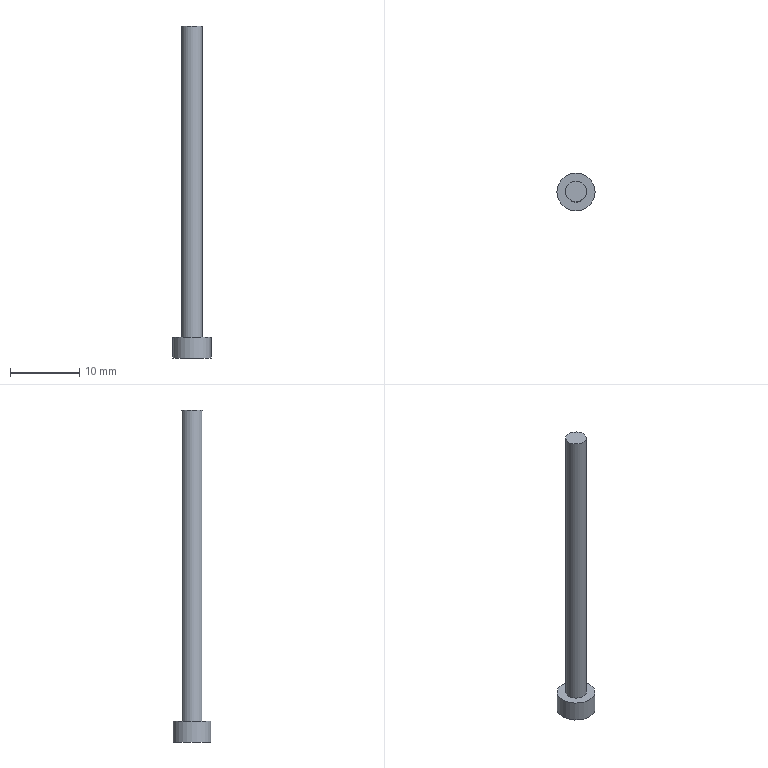Part | STEP file | 1 solid | 12 faces | box 5.5 x 5.5 x 48 mm | volume 378.644 mm3 | plane 10 | cylinder 2 | commonest cylinder face diameters 3 x1 5.5 x1
STEP:
#1=CARTESIAN_POINT('',(0.,0.,0.));
#2=DIRECTION('',(0.,0.,1.));
#3=DIRECTION('',(1.,0.,0.));
#4=AXIS2_PLACEMENT_3D('',#1,#2,#3);
#5=CARTESIAN_POINT('',(1805.407,450.23,-94.881));
#6=VERTEX_POINT('',#5);
#7=CARTESIAN_POINT('',(1808.157,450.23,-94.881));
#8=DIRECTION('',(0.,0.,-1.));
#9=DIRECTION('',(-1.,0.,0.));
#10=AXIS2_PLACEMENT_3D('',#7,#8,#9);
#11=CIRCLE('',#10,2.75);
#12=CARTESIAN_POINT('',(1805.407,450.23,-94.881));
#13=DIRECTION('',(0.,0.,1.));
#14=DIRECTION('',(1.,0.,0.));
#15=AXIS2_PLACEMENT_3D('',#12,#13,#14);
#16=PLANE('',#15);
#17=CARTESIAN_POINT('',(0.,0.));
#18=CARTESIAN_POINT('',(0.,4.763));
#19=CARTESIAN_POINT('',(4.125,2.382));
#20=CARTESIAN_POINT('',(8.25,0.));
#21=CARTESIAN_POINT('',(4.125,-2.382));
#22=CARTESIAN_POINT('',(0.,-4.763));
#23=CARTESIAN_POINT('',(0.,0.));
#24=(BOUNDED_CURVE()B_SPLINE_CURVE(2,(#17,#18,#19,#20,#21,#22,#23),.UNSPECIFIED.,.T.,.F.)B_SPLINE_CURVE_WITH_KNOTS((1,2,2,2,2,1),(-2.094,0.,2.094,4.189,6.283,8.378),.UNSPECIFIED.)CURVE()GEOMETRIC_REPRESENTATION_ITEM()RATIONAL_B_SPLINE_CURVE((1.,0.5,1.,0.5,1.,0.5,1.))REPRESENTATION_ITEM(''));
#25=(GEOMETRIC_REPRESENTATION_CONTEXT(2)PARAMETRIC_REPRESENTATION_CONTEXT()REPRESENTATION_CONTEXT('',''));
#26=DEFINITIONAL_REPRESENTATION('',(#24),#25);
#27=PCURVE('',#16,#26);
#28=CARTESIAN_POINT('',(1808.157,450.23,-52.481));
#29=DIRECTION('',(0.,0.,-1.));
#30=DIRECTION('',(-1.,0.,0.));
#31=AXIS2_PLACEMENT_3D('',#28,#29,#30);
#32=CYLINDRICAL_SURFACE('',#31,2.75);
#33=CARTESIAN_POINT('',(0.,42.4));
#34=DIRECTION('',(1.,0.));
#35=VECTOR('',#34,1.);
#36=LINE('',#33,#35);
#37=(GEOMETRIC_REPRESENTATION_CONTEXT(2)PARAMETRIC_REPRESENTATION_CONTEXT()REPRESENTATION_CONTEXT('',''));
#38=DEFINITIONAL_REPRESENTATION('',(#36),#37);
#39=PCURVE('',#32,#38);
#40=SURFACE_CURVE('',#11,(#27,#39),.PCURVE_S1.);
#41=EDGE_CURVE('',#6,#6,#40,.T.);
#42=ORIENTED_EDGE('',*,*,#41,.T.);
#43=EDGE_LOOP('',(#42));
#44=FACE_BOUND('',#43,.T.);
#45=CARTESIAN_POINT('',(1808.879,451.48,-94.881));
#46=VERTEX_POINT('',#45);
#47=CARTESIAN_POINT('',(1807.435,451.48,-94.881));
#48=VERTEX_POINT('',#47);
#49=CARTESIAN_POINT('',(1808.879,451.48,-94.881));
#50=DIRECTION('',(-1.,0.,0.));
#51=VECTOR('',#50,1.);
#52=LINE('',#49,#51);
#53=CARTESIAN_POINT('',(3.472,1.25));
#54=DIRECTION('',(-1.,0.));
#55=VECTOR('',#54,1.);
#56=LINE('',#53,#55);
#57=(GEOMETRIC_REPRESENTATION_CONTEXT(2)PARAMETRIC_REPRESENTATION_CONTEXT()REPRESENTATION_CONTEXT('',''));
#58=DEFINITIONAL_REPRESENTATION('',(#56),#57);
#59=PCURVE('',#16,#58);
#60=CARTESIAN_POINT('',(1808.879,451.48,-92.901));
#61=DIRECTION('',(0.,-1.,0.));
#62=DIRECTION('',(-1.,0.,0.));
#63=AXIS2_PLACEMENT_3D('',#60,#61,#62);
#64=PLANE('',#63);
#65=CARTESIAN_POINT('',(0.,1.98));
#66=DIRECTION('',(1.,0.));
#67=VECTOR('',#66,1.);
#68=LINE('',#65,#67);
#69=(GEOMETRIC_REPRESENTATION_CONTEXT(2)PARAMETRIC_REPRESENTATION_CONTEXT()REPRESENTATION_CONTEXT('',''));
#70=DEFINITIONAL_REPRESENTATION('',(#68),#69);
#71=PCURVE('',#64,#70);
#72=SURFACE_CURVE('',#52,(#59,#71),.PCURVE_S1.);
#73=EDGE_CURVE('',#46,#48,#72,.T.);
#74=ORIENTED_EDGE('',*,*,#73,.T.);
#75=CARTESIAN_POINT('',(1806.714,450.23,-94.881));
#76=VERTEX_POINT('',#75);
#77=CARTESIAN_POINT('',(1807.435,451.48,-94.881));
#78=DIRECTION('',(-0.5,-0.866,0.));
#79=VECTOR('',#78,1.);
#80=LINE('',#77,#79);
#81=CARTESIAN_POINT('',(2.028,1.25));
#82=DIRECTION('',(-0.5,-0.866));
#83=VECTOR('',#82,1.);
#84=LINE('',#81,#83);
#85=(GEOMETRIC_REPRESENTATION_CONTEXT(2)PARAMETRIC_REPRESENTATION_CONTEXT()REPRESENTATION_CONTEXT('',''));
#86=DEFINITIONAL_REPRESENTATION('',(#84),#85);
#87=PCURVE('',#16,#86);
#88=CARTESIAN_POINT('',(1807.435,451.48,-92.901));
#89=DIRECTION('',(0.866,-0.5,0.));
#90=DIRECTION('',(-0.5,-0.866,0.));
#91=AXIS2_PLACEMENT_3D('',#88,#89,#90);
#92=PLANE('',#91);
#93=CARTESIAN_POINT('',(0.,1.98));
#94=DIRECTION('',(1.,0.));
#95=VECTOR('',#94,1.);
#96=LINE('',#93,#95);
#97=(GEOMETRIC_REPRESENTATION_CONTEXT(2)PARAMETRIC_REPRESENTATION_CONTEXT()REPRESENTATION_CONTEXT('',''));
#98=DEFINITIONAL_REPRESENTATION('',(#96),#97);
#99=PCURVE('',#92,#98);
#100=SURFACE_CURVE('',#80,(#87,#99),.PCURVE_S1.);
#101=EDGE_CURVE('',#48,#76,#100,.T.);
#102=ORIENTED_EDGE('',*,*,#101,.T.);
#103=CARTESIAN_POINT('',(1807.435,448.98,-94.881));
#104=VERTEX_POINT('',#103);
#105=CARTESIAN_POINT('',(1806.714,450.23,-94.881));
#106=DIRECTION('',(0.5,-0.866,0.));
#107=VECTOR('',#106,1.);
#108=LINE('',#105,#107);
#109=CARTESIAN_POINT('',(1.307,0.));
#110=DIRECTION('',(0.5,-0.866));
#111=VECTOR('',#110,1.);
#112=LINE('',#109,#111);
#113=(GEOMETRIC_REPRESENTATION_CONTEXT(2)PARAMETRIC_REPRESENTATION_CONTEXT()REPRESENTATION_CONTEXT('',''));
#114=DEFINITIONAL_REPRESENTATION('',(#112),#113);
#115=PCURVE('',#16,#114);
#116=CARTESIAN_POINT('',(1806.714,450.23,-92.901));
#117=DIRECTION('',(0.866,0.5,0.));
#118=DIRECTION('',(0.5,-0.866,0.));
#119=AXIS2_PLACEMENT_3D('',#116,#117,#118);
#120=PLANE('',#119);
#121=CARTESIAN_POINT('',(0.,1.98));
#122=DIRECTION('',(1.,0.));
#123=VECTOR('',#122,1.);
#124=LINE('',#121,#123);
#125=(GEOMETRIC_REPRESENTATION_CONTEXT(2)PARAMETRIC_REPRESENTATION_CONTEXT()REPRESENTATION_CONTEXT('',''));
#126=DEFINITIONAL_REPRESENTATION('',(#124),#125);
#127=PCURVE('',#120,#126);
#128=SURFACE_CURVE('',#108,(#115,#127),.PCURVE_S1.);
#129=EDGE_CURVE('',#76,#104,#128,.T.);
#130=ORIENTED_EDGE('',*,*,#129,.T.);
#131=CARTESIAN_POINT('',(1808.879,448.98,-94.881));
#132=VERTEX_POINT('',#131);
#133=CARTESIAN_POINT('',(1807.435,448.98,-94.881));
#134=DIRECTION('',(1.,0.,0.));
#135=VECTOR('',#134,1.);
#136=LINE('',#133,#135);
#137=CARTESIAN_POINT('',(2.028,-1.25));
#138=DIRECTION('',(1.,0.));
#139=VECTOR('',#138,1.);
#140=LINE('',#137,#139);
#141=(GEOMETRIC_REPRESENTATION_CONTEXT(2)PARAMETRIC_REPRESENTATION_CONTEXT()REPRESENTATION_CONTEXT('',''));
#142=DEFINITIONAL_REPRESENTATION('',(#140),#141);
#143=PCURVE('',#16,#142);
#144=CARTESIAN_POINT('',(1807.435,448.98,-92.901));
#145=DIRECTION('',(0.,1.,0.));
#146=DIRECTION('',(1.,0.,0.));
#147=AXIS2_PLACEMENT_3D('',#144,#145,#146);
#148=PLANE('',#147);
#149=CARTESIAN_POINT('',(0.,1.98));
#150=DIRECTION('',(1.,0.));
#151=VECTOR('',#150,1.);
#152=LINE('',#149,#151);
#153=(GEOMETRIC_REPRESENTATION_CONTEXT(2)PARAMETRIC_REPRESENTATION_CONTEXT()REPRESENTATION_CONTEXT('',''));
#154=DEFINITIONAL_REPRESENTATION('',(#152),#153);
#155=PCURVE('',#148,#154);
#156=SURFACE_CURVE('',#136,(#143,#155),.PCURVE_S1.);
#157=EDGE_CURVE('',#104,#132,#156,.T.);
#158=ORIENTED_EDGE('',*,*,#157,.T.);
#159=CARTESIAN_POINT('',(1809.601,450.23,-94.881));
#160=VERTEX_POINT('',#159);
#161=CARTESIAN_POINT('',(1808.879,448.98,-94.881));
#162=DIRECTION('',(0.5,0.866,0.));
#163=VECTOR('',#162,1.);
#164=LINE('',#161,#163);
#165=CARTESIAN_POINT('',(3.472,-1.25));
#166=DIRECTION('',(0.5,0.866));
#167=VECTOR('',#166,1.);
#168=LINE('',#165,#167);
#169=(GEOMETRIC_REPRESENTATION_CONTEXT(2)PARAMETRIC_REPRESENTATION_CONTEXT()REPRESENTATION_CONTEXT('',''));
#170=DEFINITIONAL_REPRESENTATION('',(#168),#169);
#171=PCURVE('',#16,#170);
#172=CARTESIAN_POINT('',(1808.879,448.98,-92.901));
#173=DIRECTION('',(-0.866,0.5,0.));
#174=DIRECTION('',(0.5,0.866,0.));
#175=AXIS2_PLACEMENT_3D('',#172,#173,#174);
#176=PLANE('',#175);
#177=CARTESIAN_POINT('',(0.,1.98));
#178=DIRECTION('',(1.,0.));
#179=VECTOR('',#178,1.);
#180=LINE('',#177,#179);
#181=(GEOMETRIC_REPRESENTATION_CONTEXT(2)PARAMETRIC_REPRESENTATION_CONTEXT()REPRESENTATION_CONTEXT('',''));
#182=DEFINITIONAL_REPRESENTATION('',(#180),#181);
#183=PCURVE('',#176,#182);
#184=SURFACE_CURVE('',#164,(#171,#183),.PCURVE_S1.);
#185=EDGE_CURVE('',#132,#160,#184,.T.);
#186=ORIENTED_EDGE('',*,*,#185,.T.);
#187=CARTESIAN_POINT('',(1809.601,450.23,-94.881));
#188=DIRECTION('',(-0.5,0.866,0.));
#189=VECTOR('',#188,1.);
#190=LINE('',#187,#189);
#191=CARTESIAN_POINT('',(4.193,0.));
#192=DIRECTION('',(-0.5,0.866));
#193=VECTOR('',#192,1.);
#194=LINE('',#191,#193);
#195=(GEOMETRIC_REPRESENTATION_CONTEXT(2)PARAMETRIC_REPRESENTATION_CONTEXT()REPRESENTATION_CONTEXT('',''));
#196=DEFINITIONAL_REPRESENTATION('',(#194),#195);
#197=PCURVE('',#16,#196);
#198=CARTESIAN_POINT('',(1809.601,450.23,-92.901));
#199=DIRECTION('',(-0.866,-0.5,0.));
#200=DIRECTION('',(-0.5,0.866,0.));
#201=AXIS2_PLACEMENT_3D('',#198,#199,#200);
#202=PLANE('',#201);
#203=CARTESIAN_POINT('',(0.,1.98));
#204=DIRECTION('',(1.,0.));
#205=VECTOR('',#204,1.);
#206=LINE('',#203,#205);
#207=(GEOMETRIC_REPRESENTATION_CONTEXT(2)PARAMETRIC_REPRESENTATION_CONTEXT()REPRESENTATION_CONTEXT('',''));
#208=DEFINITIONAL_REPRESENTATION('',(#206),#207);
#209=PCURVE('',#202,#208);
#210=SURFACE_CURVE('',#190,(#197,#209),.PCURVE_S1.);
#211=EDGE_CURVE('',#160,#46,#210,.T.);
#212=ORIENTED_EDGE('',*,*,#211,.T.);
#213=EDGE_LOOP('',(#74,#102,#130,#158,#186,#212));
#214=FACE_BOUND('',#213,.T.);
#215=ADVANCED_FACE('',(#44,#214),#16,.F.);
#216=ORIENTED_EDGE('',*,*,#41,.F.);
#217=CARTESIAN_POINT('',(1805.407,450.23,-91.881));
#218=VERTEX_POINT('',#217);
#219=CARTESIAN_POINT('',(1805.407,450.23,-91.881));
#220=CARTESIAN_POINT('',(1805.407,450.23,-94.881));
#221=B_SPLINE_CURVE_WITH_KNOTS('',1,(#219,#220),.UNSPECIFIED.,.F.,.F.,(2,2),(39.4,42.4),.PIECEWISE_BEZIER_KNOTS.);
#222=CARTESIAN_POINT('',(0.,0.));
#223=DIRECTION('',(0.,1.));
#224=VECTOR('',#223,1.);
#225=LINE('',#222,#224);
#226=(GEOMETRIC_REPRESENTATION_CONTEXT(2)PARAMETRIC_REPRESENTATION_CONTEXT()REPRESENTATION_CONTEXT('',''));
#227=DEFINITIONAL_REPRESENTATION('',(#225),#226);
#228=PCURVE('',#32,#227);
#229=CARTESIAN_POINT('',(6.283,0.));
#230=DIRECTION('',(0.,1.));
#231=VECTOR('',#230,1.);
#232=LINE('',#229,#231);
#233=(GEOMETRIC_REPRESENTATION_CONTEXT(2)PARAMETRIC_REPRESENTATION_CONTEXT()REPRESENTATION_CONTEXT('',''));
#234=DEFINITIONAL_REPRESENTATION('',(#232),#233);
#235=PCURVE('',#32,#234);
#236=SEAM_CURVE('',#221,(#228,#235),.PCURVE_S1.);
#237=EDGE_CURVE('',#218,#6,#236,.T.);
#238=ORIENTED_EDGE('',*,*,#237,.F.);
#239=CARTESIAN_POINT('',(1808.157,450.23,-91.881));
#240=DIRECTION('',(0.,0.,-1.));
#241=DIRECTION('',(-1.,0.,0.));
#242=AXIS2_PLACEMENT_3D('',#239,#240,#241);
#243=CIRCLE('',#242,2.75);
#244=CARTESIAN_POINT('',(0.,39.4));
#245=DIRECTION('',(1.,0.));
#246=VECTOR('',#245,1.);
#247=LINE('',#244,#246);
#248=(GEOMETRIC_REPRESENTATION_CONTEXT(2)PARAMETRIC_REPRESENTATION_CONTEXT()REPRESENTATION_CONTEXT('',''));
#249=DEFINITIONAL_REPRESENTATION('',(#247),#248);
#250=PCURVE('',#32,#249);
#251=CARTESIAN_POINT('',(1806.657,450.23,-91.881));
#252=DIRECTION('',(0.,0.,-1.));
#253=DIRECTION('',(-1.,0.,0.));
#254=AXIS2_PLACEMENT_3D('',#251,#252,#253);
#255=PLANE('',#254);
#256=CARTESIAN_POINT('',(-1.5,0.));
#257=DIRECTION('',(1.,0.));
#258=AXIS2_PLACEMENT_2D('',#256,#257);
#259=CIRCLE('',#258,2.75);
#260=(GEOMETRIC_REPRESENTATION_CONTEXT(2)PARAMETRIC_REPRESENTATION_CONTEXT()REPRESENTATION_CONTEXT('',''));
#261=DEFINITIONAL_REPRESENTATION('',(#259),#260);
#262=PCURVE('',#255,#261);
#263=SURFACE_CURVE('',#243,(#250,#262),.PCURVE_S1.);
#264=EDGE_CURVE('',#218,#218,#263,.T.);
#265=ORIENTED_EDGE('',*,*,#264,.T.);
#266=ORIENTED_EDGE('',*,*,#237,.T.);
#267=EDGE_LOOP('',(#216,#238,#265,#266));
#268=FACE_BOUND('',#267,.T.);
#269=ADVANCED_FACE('',(#268),#32,.T.);
#270=ORIENTED_EDGE('',*,*,#264,.F.);
#271=EDGE_LOOP('',(#270));
#272=FACE_BOUND('',#271,.T.);
#273=CARTESIAN_POINT('',(1806.657,450.23,-91.881));
#274=VERTEX_POINT('',#273);
#275=CARTESIAN_POINT('',(1808.157,450.23,-91.881));
#276=DIRECTION('',(0.,0.,-1.));
#277=DIRECTION('',(-1.,0.,0.));
#278=AXIS2_PLACEMENT_3D('',#275,#276,#277);
#279=CIRCLE('',#278,1.5);
#280=CARTESIAN_POINT('',(-1.5,0.));
#281=DIRECTION('',(1.,0.));
#282=AXIS2_PLACEMENT_2D('',#280,#281);
#283=CIRCLE('',#282,1.5);
#284=(GEOMETRIC_REPRESENTATION_CONTEXT(2)PARAMETRIC_REPRESENTATION_CONTEXT()REPRESENTATION_CONTEXT('',''));
#285=DEFINITIONAL_REPRESENTATION('',(#283),#284);
#286=PCURVE('',#255,#285);
#287=CARTESIAN_POINT('',(1808.157,450.23,-52.481));
#288=DIRECTION('',(0.,0.,-1.));
#289=DIRECTION('',(-1.,0.,0.));
#290=AXIS2_PLACEMENT_3D('',#287,#288,#289);
#291=CYLINDRICAL_SURFACE('',#290,1.5);
#292=CARTESIAN_POINT('',(0.,39.4));
#293=DIRECTION('',(1.,0.));
#294=VECTOR('',#293,1.);
#295=LINE('',#292,#294);
#296=(GEOMETRIC_REPRESENTATION_CONTEXT(2)PARAMETRIC_REPRESENTATION_CONTEXT()REPRESENTATION_CONTEXT('',''));
#297=DEFINITIONAL_REPRESENTATION('',(#295),#296);
#298=PCURVE('',#291,#297);
#299=SURFACE_CURVE('',#279,(#286,#298),.PCURVE_S1.);
#300=EDGE_CURVE('',#274,#274,#299,.T.);
#301=ORIENTED_EDGE('',*,*,#300,.T.);
#302=EDGE_LOOP('',(#301));
#303=FACE_BOUND('',#302,.T.);
#304=ADVANCED_FACE('',(#272,#303),#255,.F.);
#305=ORIENTED_EDGE('',*,*,#300,.F.);
#306=CARTESIAN_POINT('',(1806.657,450.23,-46.881));
#307=VERTEX_POINT('',#306);
#308=CARTESIAN_POINT('',(1806.657,450.23,-46.881));
#309=CARTESIAN_POINT('',(1806.657,450.23,-91.881));
#310=B_SPLINE_CURVE_WITH_KNOTS('',1,(#308,#309),.UNSPECIFIED.,.F.,.F.,(2,2),(-5.6,39.4),.PIECEWISE_BEZIER_KNOTS.);
#311=CARTESIAN_POINT('',(0.,0.));
#312=DIRECTION('',(0.,1.));
#313=VECTOR('',#312,1.);
#314=LINE('',#311,#313);
#315=(GEOMETRIC_REPRESENTATION_CONTEXT(2)PARAMETRIC_REPRESENTATION_CONTEXT()REPRESENTATION_CONTEXT('',''));
#316=DEFINITIONAL_REPRESENTATION('',(#314),#315);
#317=PCURVE('',#291,#316);
#318=CARTESIAN_POINT('',(6.283,0.));
#319=DIRECTION('',(0.,1.));
#320=VECTOR('',#319,1.);
#321=LINE('',#318,#320);
#322=(GEOMETRIC_REPRESENTATION_CONTEXT(2)PARAMETRIC_REPRESENTATION_CONTEXT()REPRESENTATION_CONTEXT('',''));
#323=DEFINITIONAL_REPRESENTATION('',(#321),#322);
#324=PCURVE('',#291,#323);
#325=SEAM_CURVE('',#310,(#317,#324),.PCURVE_S1.);
#326=EDGE_CURVE('',#307,#274,#325,.T.);
#327=ORIENTED_EDGE('',*,*,#326,.F.);
#328=CARTESIAN_POINT('',(1808.157,450.23,-46.881));
#329=DIRECTION('',(0.,0.,-1.));
#330=DIRECTION('',(-1.,0.,0.));
#331=AXIS2_PLACEMENT_3D('',#328,#329,#330);
#332=CIRCLE('',#331,1.5);
#333=CARTESIAN_POINT('',(0.,-5.6));
#334=DIRECTION('',(1.,0.));
#335=VECTOR('',#334,1.);
#336=LINE('',#333,#335);
#337=(GEOMETRIC_REPRESENTATION_CONTEXT(2)PARAMETRIC_REPRESENTATION_CONTEXT()REPRESENTATION_CONTEXT('',''));
#338=DEFINITIONAL_REPRESENTATION('',(#336),#337);
#339=PCURVE('',#291,#338);
#340=CARTESIAN_POINT('',(1808.157,450.23,-46.881));
#341=DIRECTION('',(0.,0.,-1.));
#342=DIRECTION('',(-1.,0.,0.));
#343=AXIS2_PLACEMENT_3D('',#340,#341,#342);
#344=PLANE('',#343);
#345=CARTESIAN_POINT('',(0.,0.));
#346=DIRECTION('',(1.,0.));
#347=AXIS2_PLACEMENT_2D('',#345,#346);
#348=CIRCLE('',#347,1.5);
#349=(GEOMETRIC_REPRESENTATION_CONTEXT(2)PARAMETRIC_REPRESENTATION_CONTEXT()REPRESENTATION_CONTEXT('',''));
#350=DEFINITIONAL_REPRESENTATION('',(#348),#349);
#351=PCURVE('',#344,#350);
#352=SURFACE_CURVE('',#332,(#339,#351),.PCURVE_S1.);
#353=EDGE_CURVE('',#307,#307,#352,.T.);
#354=ORIENTED_EDGE('',*,*,#353,.T.);
#355=ORIENTED_EDGE('',*,*,#326,.T.);
#356=EDGE_LOOP('',(#305,#327,#354,#355));
#357=FACE_BOUND('',#356,.T.);
#358=ADVANCED_FACE('',(#357),#291,.T.);
#359=ORIENTED_EDGE('',*,*,#353,.F.);
#360=EDGE_LOOP('',(#359));
#361=FACE_BOUND('',#360,.T.);
#362=ADVANCED_FACE('',(#361),#344,.F.);
#363=ORIENTED_EDGE('',*,*,#73,.F.);
#364=CARTESIAN_POINT('',(1808.879,451.48,-92.901));
#365=VERTEX_POINT('',#364);
#366=CARTESIAN_POINT('',(1808.879,451.48,-92.901));
#367=DIRECTION('',(0.,0.,1.));
#368=VECTOR('',#367,1.);
#369=LINE('',#366,#368);
#370=CARTESIAN_POINT('',(0.,0.));
#371=DIRECTION('',(0.,-1.));
#372=VECTOR('',#371,1.);
#373=LINE('',#370,#372);
#374=(GEOMETRIC_REPRESENTATION_CONTEXT(2)PARAMETRIC_REPRESENTATION_CONTEXT()REPRESENTATION_CONTEXT('',''));
#375=DEFINITIONAL_REPRESENTATION('',(#373),#374);
#376=PCURVE('',#64,#375);
#377=CARTESIAN_POINT('',(1.443,0.));
#378=DIRECTION('',(0.,-1.));
#379=VECTOR('',#378,1.);
#380=LINE('',#377,#379);
#381=(GEOMETRIC_REPRESENTATION_CONTEXT(2)PARAMETRIC_REPRESENTATION_CONTEXT()REPRESENTATION_CONTEXT('',''));
#382=DEFINITIONAL_REPRESENTATION('',(#380),#381);
#383=PCURVE('',#202,#382);
#384=SURFACE_CURVE('',#369,(#376,#383),.PCURVE_S1.);
#385=EDGE_CURVE('',#46,#365,#384,.T.);
#386=ORIENTED_EDGE('',*,*,#385,.T.);
#387=CARTESIAN_POINT('',(1807.435,451.48,-92.901));
#388=VERTEX_POINT('',#387);
#389=CARTESIAN_POINT('',(1808.879,451.48,-92.901));
#390=DIRECTION('',(1.,0.,0.));
#391=VECTOR('',#390,1.);
#392=LINE('',#389,#391);
#393=CARTESIAN_POINT('',(0.,0.));
#394=DIRECTION('',(-1.,0.));
#395=VECTOR('',#394,1.);
#396=LINE('',#393,#395);
#397=(GEOMETRIC_REPRESENTATION_CONTEXT(2)PARAMETRIC_REPRESENTATION_CONTEXT()REPRESENTATION_CONTEXT('',''));
#398=DEFINITIONAL_REPRESENTATION('',(#396),#397);
#399=PCURVE('',#64,#398);
#400=CARTESIAN_POINT('',(1808.157,450.23,-92.901));
#401=DIRECTION('',(0.,0.,1.));
#402=DIRECTION('',(1.,0.,0.));
#403=AXIS2_PLACEMENT_3D('',#400,#401,#402);
#404=PLANE('',#403);
#405=CARTESIAN_POINT('',(0.7217,1.25));
#406=DIRECTION('',(1.,0.));
#407=VECTOR('',#406,1.);
#408=LINE('',#405,#407);
#409=(GEOMETRIC_REPRESENTATION_CONTEXT(2)PARAMETRIC_REPRESENTATION_CONTEXT()REPRESENTATION_CONTEXT('',''));
#410=DEFINITIONAL_REPRESENTATION('',(#408),#409);
#411=PCURVE('',#404,#410);
#412=SURFACE_CURVE('',#392,(#399,#411),.PCURVE_S1.);
#413=EDGE_CURVE('',#388,#365,#412,.T.);
#414=ORIENTED_EDGE('',*,*,#413,.F.);
#415=CARTESIAN_POINT('',(1807.435,451.48,-92.901));
#416=DIRECTION('',(0.,0.,1.));
#417=VECTOR('',#416,1.);
#418=LINE('',#415,#417);
#419=CARTESIAN_POINT('',(1.443,0.));
#420=DIRECTION('',(0.,-1.));
#421=VECTOR('',#420,1.);
#422=LINE('',#419,#421);
#423=(GEOMETRIC_REPRESENTATION_CONTEXT(2)PARAMETRIC_REPRESENTATION_CONTEXT()REPRESENTATION_CONTEXT('',''));
#424=DEFINITIONAL_REPRESENTATION('',(#422),#423);
#425=PCURVE('',#64,#424);
#426=CARTESIAN_POINT('',(0.,0.));
#427=DIRECTION('',(0.,-1.));
#428=VECTOR('',#427,1.);
#429=LINE('',#426,#428);
#430=(GEOMETRIC_REPRESENTATION_CONTEXT(2)PARAMETRIC_REPRESENTATION_CONTEXT()REPRESENTATION_CONTEXT('',''));
#431=DEFINITIONAL_REPRESENTATION('',(#429),#430);
#432=PCURVE('',#92,#431);
#433=SURFACE_CURVE('',#418,(#425,#432),.PCURVE_S1.);
#434=EDGE_CURVE('',#48,#388,#433,.T.);
#435=ORIENTED_EDGE('',*,*,#434,.F.);
#436=EDGE_LOOP('',(#363,#386,#414,#435));
#437=FACE_BOUND('',#436,.T.);
#438=ADVANCED_FACE('',(#437),#64,.T.);
#439=ORIENTED_EDGE('',*,*,#101,.F.);
#440=ORIENTED_EDGE('',*,*,#434,.T.);
#441=CARTESIAN_POINT('',(1806.714,450.23,-92.901));
#442=VERTEX_POINT('',#441);
#443=CARTESIAN_POINT('',(1807.435,451.48,-92.901));
#444=DIRECTION('',(0.5,0.866,0.));
#445=VECTOR('',#444,1.);
#446=LINE('',#443,#445);
#447=CARTESIAN_POINT('',(0.,0.));
#448=DIRECTION('',(-1.,0.));
#449=VECTOR('',#448,1.);
#450=LINE('',#447,#449);
#451=(GEOMETRIC_REPRESENTATION_CONTEXT(2)PARAMETRIC_REPRESENTATION_CONTEXT()REPRESENTATION_CONTEXT('',''));
#452=DEFINITIONAL_REPRESENTATION('',(#450),#451);
#453=PCURVE('',#92,#452);
#454=CARTESIAN_POINT('',(-0.7217,1.25));
#455=DIRECTION('',(0.5,0.866));
#456=VECTOR('',#455,1.);
#457=LINE('',#454,#456);
#458=(GEOMETRIC_REPRESENTATION_CONTEXT(2)PARAMETRIC_REPRESENTATION_CONTEXT()REPRESENTATION_CONTEXT('',''));
#459=DEFINITIONAL_REPRESENTATION('',(#457),#458);
#460=PCURVE('',#404,#459);
#461=SURFACE_CURVE('',#446,(#453,#460),.PCURVE_S1.);
#462=EDGE_CURVE('',#442,#388,#461,.T.);
#463=ORIENTED_EDGE('',*,*,#462,.F.);
#464=CARTESIAN_POINT('',(1806.714,450.23,-92.901));
#465=DIRECTION('',(0.,0.,1.));
#466=VECTOR('',#465,1.);
#467=LINE('',#464,#466);
#468=CARTESIAN_POINT('',(1.443,0.));
#469=DIRECTION('',(0.,-1.));
#470=VECTOR('',#469,1.);
#471=LINE('',#468,#470);
#472=(GEOMETRIC_REPRESENTATION_CONTEXT(2)PARAMETRIC_REPRESENTATION_CONTEXT()REPRESENTATION_CONTEXT('',''));
#473=DEFINITIONAL_REPRESENTATION('',(#471),#472);
#474=PCURVE('',#92,#473);
#475=CARTESIAN_POINT('',(0.,0.));
#476=DIRECTION('',(0.,-1.));
#477=VECTOR('',#476,1.);
#478=LINE('',#475,#477);
#479=(GEOMETRIC_REPRESENTATION_CONTEXT(2)PARAMETRIC_REPRESENTATION_CONTEXT()REPRESENTATION_CONTEXT('',''));
#480=DEFINITIONAL_REPRESENTATION('',(#478),#479);
#481=PCURVE('',#120,#480);
#482=SURFACE_CURVE('',#467,(#474,#481),.PCURVE_S1.);
#483=EDGE_CURVE('',#76,#442,#482,.T.);
#484=ORIENTED_EDGE('',*,*,#483,.F.);
#485=EDGE_LOOP('',(#439,#440,#463,#484));
#486=FACE_BOUND('',#485,.T.);
#487=ADVANCED_FACE('',(#486),#92,.T.);
#488=ORIENTED_EDGE('',*,*,#129,.F.);
#489=ORIENTED_EDGE('',*,*,#483,.T.);
#490=CARTESIAN_POINT('',(1807.435,448.98,-92.901));
#491=VERTEX_POINT('',#490);
#492=CARTESIAN_POINT('',(1806.714,450.23,-92.901));
#493=DIRECTION('',(-0.5,0.866,0.));
#494=VECTOR('',#493,1.);
#495=LINE('',#492,#494);
#496=CARTESIAN_POINT('',(0.,0.));
#497=DIRECTION('',(-1.,0.));
#498=VECTOR('',#497,1.);
#499=LINE('',#496,#498);
#500=(GEOMETRIC_REPRESENTATION_CONTEXT(2)PARAMETRIC_REPRESENTATION_CONTEXT()REPRESENTATION_CONTEXT('',''));
#501=DEFINITIONAL_REPRESENTATION('',(#499),#500);
#502=PCURVE('',#120,#501);
#503=CARTESIAN_POINT('',(-1.443,0.));
#504=DIRECTION('',(-0.5,0.866));
#505=VECTOR('',#504,1.);
#506=LINE('',#503,#505);
#507=(GEOMETRIC_REPRESENTATION_CONTEXT(2)PARAMETRIC_REPRESENTATION_CONTEXT()REPRESENTATION_CONTEXT('',''));
#508=DEFINITIONAL_REPRESENTATION('',(#506),#507);
#509=PCURVE('',#404,#508);
#510=SURFACE_CURVE('',#495,(#502,#509),.PCURVE_S1.);
#511=EDGE_CURVE('',#491,#442,#510,.T.);
#512=ORIENTED_EDGE('',*,*,#511,.F.);
#513=CARTESIAN_POINT('',(1807.435,448.98,-92.901));
#514=DIRECTION('',(0.,0.,1.));
#515=VECTOR('',#514,1.);
#516=LINE('',#513,#515);
#517=CARTESIAN_POINT('',(1.443,0.));
#518=DIRECTION('',(0.,-1.));
#519=VECTOR('',#518,1.);
#520=LINE('',#517,#519);
#521=(GEOMETRIC_REPRESENTATION_CONTEXT(2)PARAMETRIC_REPRESENTATION_CONTEXT()REPRESENTATION_CONTEXT('',''));
#522=DEFINITIONAL_REPRESENTATION('',(#520),#521);
#523=PCURVE('',#120,#522);
#524=CARTESIAN_POINT('',(0.,0.));
#525=DIRECTION('',(0.,-1.));
#526=VECTOR('',#525,1.);
#527=LINE('',#524,#526);
#528=(GEOMETRIC_REPRESENTATION_CONTEXT(2)PARAMETRIC_REPRESENTATION_CONTEXT()REPRESENTATION_CONTEXT('',''));
#529=DEFINITIONAL_REPRESENTATION('',(#527),#528);
#530=PCURVE('',#148,#529);
#531=SURFACE_CURVE('',#516,(#523,#530),.PCURVE_S1.);
#532=EDGE_CURVE('',#104,#491,#531,.T.);
#533=ORIENTED_EDGE('',*,*,#532,.F.);
#534=EDGE_LOOP('',(#488,#489,#512,#533));
#535=FACE_BOUND('',#534,.T.);
#536=ADVANCED_FACE('',(#535),#120,.T.);
#537=ORIENTED_EDGE('',*,*,#157,.F.);
#538=ORIENTED_EDGE('',*,*,#532,.T.);
#539=CARTESIAN_POINT('',(1808.879,448.98,-92.901));
#540=VERTEX_POINT('',#539);
#541=CARTESIAN_POINT('',(1807.435,448.98,-92.901));
#542=DIRECTION('',(-1.,0.,0.));
#543=VECTOR('',#542,1.);
#544=LINE('',#541,#543);
#545=CARTESIAN_POINT('',(0.,0.));
#546=DIRECTION('',(-1.,0.));
#547=VECTOR('',#546,1.);
#548=LINE('',#545,#547);
#549=(GEOMETRIC_REPRESENTATION_CONTEXT(2)PARAMETRIC_REPRESENTATION_CONTEXT()REPRESENTATION_CONTEXT('',''));
#550=DEFINITIONAL_REPRESENTATION('',(#548),#549);
#551=PCURVE('',#148,#550);
#552=CARTESIAN_POINT('',(-0.7217,-1.25));
#553=DIRECTION('',(-1.,0.));
#554=VECTOR('',#553,1.);
#555=LINE('',#552,#554);
#556=(GEOMETRIC_REPRESENTATION_CONTEXT(2)PARAMETRIC_REPRESENTATION_CONTEXT()REPRESENTATION_CONTEXT('',''));
#557=DEFINITIONAL_REPRESENTATION('',(#555),#556);
#558=PCURVE('',#404,#557);
#559=SURFACE_CURVE('',#544,(#551,#558),.PCURVE_S1.);
#560=EDGE_CURVE('',#540,#491,#559,.T.);
#561=ORIENTED_EDGE('',*,*,#560,.F.);
#562=CARTESIAN_POINT('',(1808.879,448.98,-92.901));
#563=DIRECTION('',(0.,0.,1.));
#564=VECTOR('',#563,1.);
#565=LINE('',#562,#564);
#566=CARTESIAN_POINT('',(1.443,0.));
#567=DIRECTION('',(0.,-1.));
#568=VECTOR('',#567,1.);
#569=LINE('',#566,#568);
#570=(GEOMETRIC_REPRESENTATION_CONTEXT(2)PARAMETRIC_REPRESENTATION_CONTEXT()REPRESENTATION_CONTEXT('',''));
#571=DEFINITIONAL_REPRESENTATION('',(#569),#570);
#572=PCURVE('',#148,#571);
#573=CARTESIAN_POINT('',(0.,0.));
#574=DIRECTION('',(0.,-1.));
#575=VECTOR('',#574,1.);
#576=LINE('',#573,#575);
#577=(GEOMETRIC_REPRESENTATION_CONTEXT(2)PARAMETRIC_REPRESENTATION_CONTEXT()REPRESENTATION_CONTEXT('',''));
#578=DEFINITIONAL_REPRESENTATION('',(#576),#577);
#579=PCURVE('',#176,#578);
#580=SURFACE_CURVE('',#565,(#572,#579),.PCURVE_S1.);
#581=EDGE_CURVE('',#132,#540,#580,.T.);
#582=ORIENTED_EDGE('',*,*,#581,.F.);
#583=EDGE_LOOP('',(#537,#538,#561,#582));
#584=FACE_BOUND('',#583,.T.);
#585=ADVANCED_FACE('',(#584),#148,.T.);
#586=ORIENTED_EDGE('',*,*,#185,.F.);
#587=ORIENTED_EDGE('',*,*,#581,.T.);
#588=CARTESIAN_POINT('',(1809.601,450.23,-92.901));
#589=VERTEX_POINT('',#588);
#590=CARTESIAN_POINT('',(1808.879,448.98,-92.901));
#591=DIRECTION('',(-0.5,-0.866,0.));
#592=VECTOR('',#591,1.);
#593=LINE('',#590,#592);
#594=CARTESIAN_POINT('',(0.,0.));
#595=DIRECTION('',(-1.,0.));
#596=VECTOR('',#595,1.);
#597=LINE('',#594,#596);
#598=(GEOMETRIC_REPRESENTATION_CONTEXT(2)PARAMETRIC_REPRESENTATION_CONTEXT()REPRESENTATION_CONTEXT('',''));
#599=DEFINITIONAL_REPRESENTATION('',(#597),#598);
#600=PCURVE('',#176,#599);
#601=CARTESIAN_POINT('',(0.7217,-1.25));
#602=DIRECTION('',(-0.5,-0.866));
#603=VECTOR('',#602,1.);
#604=LINE('',#601,#603);
#605=(GEOMETRIC_REPRESENTATION_CONTEXT(2)PARAMETRIC_REPRESENTATION_CONTEXT()REPRESENTATION_CONTEXT('',''));
#606=DEFINITIONAL_REPRESENTATION('',(#604),#605);
#607=PCURVE('',#404,#606);
#608=SURFACE_CURVE('',#593,(#600,#607),.PCURVE_S1.);
#609=EDGE_CURVE('',#589,#540,#608,.T.);
#610=ORIENTED_EDGE('',*,*,#609,.F.);
#611=CARTESIAN_POINT('',(1809.601,450.23,-92.901));
#612=DIRECTION('',(0.,0.,1.));
#613=VECTOR('',#612,1.);
#614=LINE('',#611,#613);
#615=CARTESIAN_POINT('',(1.443,0.));
#616=DIRECTION('',(0.,-1.));
#617=VECTOR('',#616,1.);
#618=LINE('',#615,#617);
#619=(GEOMETRIC_REPRESENTATION_CONTEXT(2)PARAMETRIC_REPRESENTATION_CONTEXT()REPRESENTATION_CONTEXT('',''));
#620=DEFINITIONAL_REPRESENTATION('',(#618),#619);
#621=PCURVE('',#176,#620);
#622=CARTESIAN_POINT('',(0.,0.));
#623=DIRECTION('',(0.,-1.));
#624=VECTOR('',#623,1.);
#625=LINE('',#622,#624);
#626=(GEOMETRIC_REPRESENTATION_CONTEXT(2)PARAMETRIC_REPRESENTATION_CONTEXT()REPRESENTATION_CONTEXT('',''));
#627=DEFINITIONAL_REPRESENTATION('',(#625),#626);
#628=PCURVE('',#202,#627);
#629=SURFACE_CURVE('',#614,(#621,#628),.PCURVE_S1.);
#630=EDGE_CURVE('',#160,#589,#629,.T.);
#631=ORIENTED_EDGE('',*,*,#630,.F.);
#632=EDGE_LOOP('',(#586,#587,#610,#631));
#633=FACE_BOUND('',#632,.T.);
#634=ADVANCED_FACE('',(#633),#176,.T.);
#635=ORIENTED_EDGE('',*,*,#211,.F.);
#636=ORIENTED_EDGE('',*,*,#630,.T.);
#637=CARTESIAN_POINT('',(1809.601,450.23,-92.901));
#638=DIRECTION('',(0.5,-0.866,0.));
#639=VECTOR('',#638,1.);
#640=LINE('',#637,#639);
#641=CARTESIAN_POINT('',(0.,0.));
#642=DIRECTION('',(-1.,0.));
#643=VECTOR('',#642,1.);
#644=LINE('',#641,#643);
#645=(GEOMETRIC_REPRESENTATION_CONTEXT(2)PARAMETRIC_REPRESENTATION_CONTEXT()REPRESENTATION_CONTEXT('',''));
#646=DEFINITIONAL_REPRESENTATION('',(#644),#645);
#647=PCURVE('',#202,#646);
#648=CARTESIAN_POINT('',(1.443,0.));
#649=DIRECTION('',(0.5,-0.866));
#650=VECTOR('',#649,1.);
#651=LINE('',#648,#650);
#652=(GEOMETRIC_REPRESENTATION_CONTEXT(2)PARAMETRIC_REPRESENTATION_CONTEXT()REPRESENTATION_CONTEXT('',''));
#653=DEFINITIONAL_REPRESENTATION('',(#651),#652);
#654=PCURVE('',#404,#653);
#655=SURFACE_CURVE('',#640,(#647,#654),.PCURVE_S1.);
#656=EDGE_CURVE('',#365,#589,#655,.T.);
#657=ORIENTED_EDGE('',*,*,#656,.F.);
#658=ORIENTED_EDGE('',*,*,#385,.F.);
#659=EDGE_LOOP('',(#635,#636,#657,#658));
#660=FACE_BOUND('',#659,.T.);
#661=ADVANCED_FACE('',(#660),#202,.T.);
#662=ORIENTED_EDGE('',*,*,#413,.T.);
#663=ORIENTED_EDGE('',*,*,#656,.T.);
#664=ORIENTED_EDGE('',*,*,#609,.T.);
#665=ORIENTED_EDGE('',*,*,#560,.T.);
#666=ORIENTED_EDGE('',*,*,#511,.T.);
#667=ORIENTED_EDGE('',*,*,#462,.T.);
#668=EDGE_LOOP('',(#662,#663,#664,#665,#666,#667));
#669=FACE_BOUND('',#668,.T.);
#670=ADVANCED_FACE('',(#669),#404,.F.);
#671=CLOSED_SHELL('',(#215,#269,#304,#358,#362,#438,#487,#536,#585,#634,#661,#670));
#672=MANIFOLD_SOLID_BREP('',#671);
#673=(LENGTH_UNIT()NAMED_UNIT(*)SI_UNIT(.MILLI.,.METRE.));
#674=UNCERTAINTY_MEASURE_WITH_UNIT(LENGTH_MEASURE(0.000002),#673,'','');
#675=(NAMED_UNIT(*)PLANE_ANGLE_UNIT()SI_UNIT($,.RADIAN.));
#676=(NAMED_UNIT(*)SI_UNIT($,.STERADIAN.)SOLID_ANGLE_UNIT());
#677=(GEOMETRIC_REPRESENTATION_CONTEXT(3)GLOBAL_UNCERTAINTY_ASSIGNED_CONTEXT((#674))GLOBAL_UNIT_ASSIGNED_CONTEXT((#673,#675,#676))REPRESENTATION_CONTEXT('',''));
#678=ADVANCED_BREP_SHAPE_REPRESENTATION('',(#4,#672),#677);